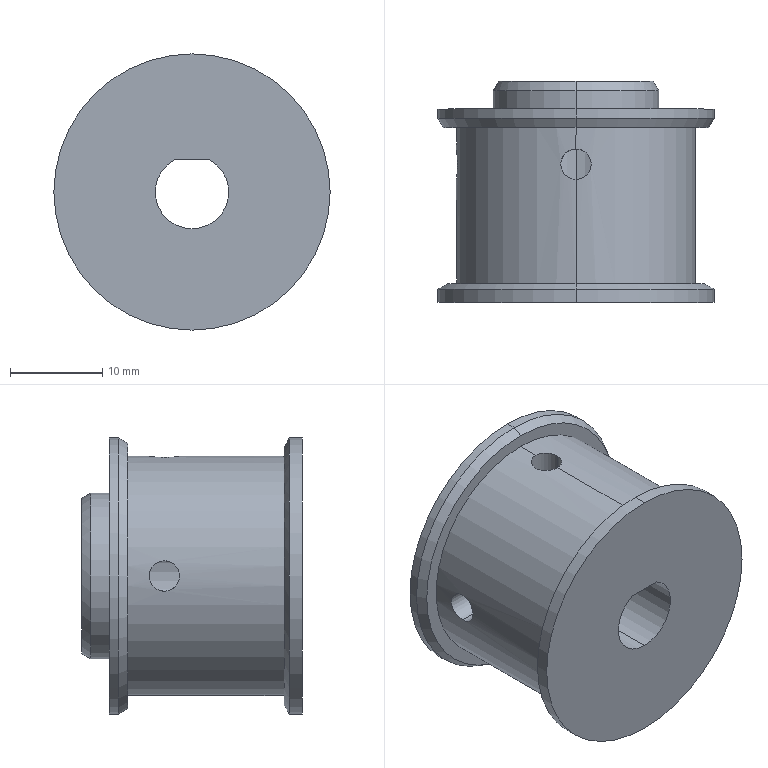Part | SolidWorks | features ICE 11, Chamfer 4, CirPattern 1, HoleWzd 1, Revolution 1 | 1 solid | 26 faces | box 30 x 24 x 30 mm | volume 11200 mm3 | cylinder 14 | cone 6 | plane 6 | commonest cylinder face diameters 3.3 x4 30 x4 8 x2 18 x2 25.98 x2
STEP:
#1=CARTESIAN_POINT('',(0.,24.,8.423));
#2=VERTEX_POINT('',#1);
#3=CARTESIAN_POINT('',(0.,24.,-8.423));
#4=VERTEX_POINT('',#3);
#5=CARTESIAN_POINT('',(0.,24.,0.));
#6=DIRECTION('',(0.,1.,0.));
#7=DIRECTION('',(0.,0.,1.));
#8=AXIS2_PLACEMENT_3D('',#5,#6,#7);
#9=CIRCLE('',#8,8.423);
#10=EDGE_CURVE('',#2,#4,#9,.T.);
#11=ORIENTED_EDGE('',*,*,#10,.F.);
#12=CARTESIAN_POINT('',(0.,23.,9.));
#13=VERTEX_POINT('',#12);
#14=CARTESIAN_POINT('',(0.,24.,8.423));
#15=DIRECTION('',(0.,-0.866,0.5));
#16=VECTOR('',#15,1000.);
#17=LINE('',#14,#16);
#18=EDGE_CURVE('',#2,#13,#17,.T.);
#19=ORIENTED_EDGE('',*,*,#18,.T.);
#20=CARTESIAN_POINT('',(0.,23.,-9.));
#21=VERTEX_POINT('',#20);
#22=CARTESIAN_POINT('',(0.,23.,0.));
#23=DIRECTION('',(0.,-1.,0.));
#24=DIRECTION('',(0.,0.,1.));
#25=AXIS2_PLACEMENT_3D('',#22,#23,#24);
#26=CIRCLE('',#25,9.);
#27=EDGE_CURVE('',#21,#13,#26,.T.);
#28=ORIENTED_EDGE('',*,*,#27,.F.);
#29=CARTESIAN_POINT('',(0.,24.,-8.423));
#30=DIRECTION('',(0.,-0.866,-0.5));
#31=VECTOR('',#30,1000.);
#32=LINE('',#29,#31);
#33=EDGE_CURVE('',#4,#21,#32,.T.);
#34=ORIENTED_EDGE('',*,*,#33,.F.);
#35=EDGE_LOOP('',(#11,#19,#28,#34));
#36=FACE_OUTER_BOUND('',#35,.T.);
#37=CARTESIAN_POINT('',(0.,24.,0.));
#38=DIRECTION('',(0.,-1.,0.));
#39=DIRECTION('',(0.,0.,-1.));
#40=AXIS2_PLACEMENT_3D('',#37,#38,#39);
#41=CONICAL_SURFACE('',#40,8.423,0.5236);
#42=ADVANCED_FACE('',(#36),#41,.T.);
#43=CARTESIAN_POINT('',(-12.885,15.,-1.65));
#44=VERTEX_POINT('',#43);
#45=CARTESIAN_POINT('',(-12.885,15.,1.65));
#46=VERTEX_POINT('',#45);
#47=CARTESIAN_POINT('',(-12.885,15.,-1.65));
#48=CARTESIAN_POINT('',(-12.885,14.891,-1.65));
#49=CARTESIAN_POINT('',(-12.886,14.784,-1.639));
#50=CARTESIAN_POINT('',(-12.891,14.573,-1.597));
#51=CARTESIAN_POINT('',(-12.895,14.468,-1.566));
#52=CARTESIAN_POINT('',(-12.905,14.268,-1.483));
#53=CARTESIAN_POINT('',(-12.911,14.173,-1.432));
#54=CARTESIAN_POINT('',(-12.924,13.994,-1.312));
#55=CARTESIAN_POINT('',(-12.931,13.909,-1.243));
#56=CARTESIAN_POINT('',(-12.951,13.681,-1.014));
#57=CARTESIAN_POINT('',(-12.965,13.558,-0.8305));
#58=CARTESIAN_POINT('',(-12.984,13.393,-0.4334));
#59=CARTESIAN_POINT('',(-12.99,13.35,-0.2161));
#60=CARTESIAN_POINT('',(-12.99,13.35,0.1071));
#61=CARTESIAN_POINT('',(-12.989,13.361,0.2166));
#62=CARTESIAN_POINT('',(-12.983,13.403,0.4283));
#63=CARTESIAN_POINT('',(-12.98,13.434,0.5312));
#64=CARTESIAN_POINT('',(-12.97,13.517,0.7311));
#65=CARTESIAN_POINT('',(-12.964,13.569,0.8276));
#66=CARTESIAN_POINT('',(-12.951,13.688,1.006));
#67=CARTESIAN_POINT('',(-12.944,13.756,1.09));
#68=CARTESIAN_POINT('',(-12.931,13.91,1.244));
#69=CARTESIAN_POINT('',(-12.924,13.993,1.312));
#70=CARTESIAN_POINT('',(-12.911,14.172,1.431));
#71=CARTESIAN_POINT('',(-12.905,14.269,1.483));
#72=CARTESIAN_POINT('',(-12.895,14.468,1.566));
#73=CARTESIAN_POINT('',(-12.891,14.571,1.597));
#74=CARTESIAN_POINT('',(-12.886,14.783,1.639));
#75=CARTESIAN_POINT('',(-12.885,14.892,1.65));
#76=CARTESIAN_POINT('',(-12.885,15.,1.65));
#77=B_SPLINE_CURVE_WITH_KNOTS('',3,(#47,#48,#49,#50,#51,#52,#53,#54,#55,#56,#57,#58,#59,#60,#61,#62,#63,#64,#65,#66,#67,#68,#69,#70,#71,#72,#73,#74,#75,#76),.UNSPECIFIED.,.F.,.F.,(4,2,2,2,2,2,2,2,2,2,2,2,2,2,4),(0.,0.0003227,0.0006455,0.0009682,0.001291,0.001936,0.002582,0.002905,0.003227,0.00355,0.003873,0.004196,0.004518,0.004841,0.005164),.UNSPECIFIED.);
#78=EDGE_CURVE('',#44,#46,#77,.T.);
#79=ORIENTED_EDGE('',*,*,#78,.T.);
#80=CARTESIAN_POINT('',(-3.644,15.,1.65));
#81=VERTEX_POINT('',#80);
#82=CARTESIAN_POINT('',(0.,15.,1.65));
#83=DIRECTION('',(1.,0.,0.));
#84=VECTOR('',#83,1000.);
#85=LINE('',#82,#84);
#86=EDGE_CURVE('',#46,#81,#85,.T.);
#87=ORIENTED_EDGE('',*,*,#86,.T.);
#88=CARTESIAN_POINT('',(-3.644,15.,-1.65));
#89=VERTEX_POINT('',#88);
#90=CARTESIAN_POINT('',(-3.644,15.,1.65));
#91=CARTESIAN_POINT('',(-3.644,14.891,1.65));
#92=CARTESIAN_POINT('',(-3.649,14.781,1.639));
#93=CARTESIAN_POINT('',(-3.668,14.568,1.596));
#94=CARTESIAN_POINT('',(-3.682,14.464,1.564));
#95=CARTESIAN_POINT('',(-3.733,14.165,1.439));
#96=CARTESIAN_POINT('',(-3.78,13.985,1.318));
#97=CARTESIAN_POINT('',(-3.849,13.757,1.091));
#98=CARTESIAN_POINT('',(-3.872,13.69,1.008));
#99=CARTESIAN_POINT('',(-3.914,13.571,0.8311));
#100=CARTESIAN_POINT('',(-3.933,13.519,0.7348));
#101=CARTESIAN_POINT('',(-3.965,13.436,0.5356));
#102=CARTESIAN_POINT('',(-3.978,13.404,0.4326));
#103=CARTESIAN_POINT('',(-3.995,13.361,0.2196));
#104=CARTESIAN_POINT('',(-4.,13.35,0.109));
#105=CARTESIAN_POINT('',(-4.,13.35,-0.2173));
#106=CARTESIAN_POINT('',(-3.981,13.394,-0.4365));
#107=CARTESIAN_POINT('',(-3.933,13.519,-0.7349));
#108=CARTESIAN_POINT('',(-3.914,13.571,-0.8311));
#109=CARTESIAN_POINT('',(-3.872,13.69,-1.009));
#110=CARTESIAN_POINT('',(-3.849,13.758,-1.091));
#111=CARTESIAN_POINT('',(-3.803,13.909,-1.243));
#112=CARTESIAN_POINT('',(-3.78,13.993,-1.311));
#113=CARTESIAN_POINT('',(-3.736,14.17,-1.43));
#114=CARTESIAN_POINT('',(-3.716,14.264,-1.481));
#115=CARTESIAN_POINT('',(-3.664,14.565,-1.607));
#116=CARTESIAN_POINT('',(-3.644,14.779,-1.65));
#117=CARTESIAN_POINT('',(-3.644,15.,-1.65));
#118=B_SPLINE_CURVE_WITH_KNOTS('',3,(#90,#91,#92,#93,#94,#95,#96,#97,#98,#99,#100,#101,#102,#103,#104,#105,#106,#107,#108,#109,#110,#111,#112,#113,#114,#115,#116,#117),.UNSPECIFIED.,.F.,.F.,(4,2,2,2,2,2,2,2,2,2,2,2,2,4),(0.005217,0.005543,0.005869,0.006521,0.006846,0.007172,0.007498,0.007824,0.008476,0.008801,0.009127,0.009453,0.009779,0.01043),.UNSPECIFIED.);
#119=EDGE_CURVE('',#81,#89,#118,.T.);
#120=ORIENTED_EDGE('',*,*,#119,.T.);
#121=CARTESIAN_POINT('',(0.,15.,-1.65));
#122=DIRECTION('',(1.,0.,0.));
#123=VECTOR('',#122,1000.);
#124=LINE('',#121,#123);
#125=EDGE_CURVE('',#44,#89,#124,.T.);
#126=ORIENTED_EDGE('',*,*,#125,.F.);
#127=EDGE_LOOP('',(#79,#87,#120,#126));
#128=FACE_OUTER_BOUND('',#127,.T.);
#129=CARTESIAN_POINT('',(0.,15.,0.));
#130=DIRECTION('',(1.,0.,0.));
#131=DIRECTION('',(0.,0.,-1.));
#132=AXIS2_PLACEMENT_3D('',#129,#130,#131);
#133=CYLINDRICAL_SURFACE('',#132,1.65);
#134=ADVANCED_FACE('',(#128),#133,.F.);
#135=CARTESIAN_POINT('',(0.,13.35,12.99));
#136=VERTEX_POINT('',#135);
#137=CARTESIAN_POINT('',(1.65,15.,12.885));
#138=VERTEX_POINT('',#137);
#139=CARTESIAN_POINT('',(0.,13.35,12.99));
#140=CARTESIAN_POINT('',(0.1077,13.35,12.99));
#141=CARTESIAN_POINT('',(0.2171,13.361,12.989));
#142=CARTESIAN_POINT('',(0.4288,13.403,12.983));
#143=CARTESIAN_POINT('',(0.5317,13.434,12.98));
#144=CARTESIAN_POINT('',(0.7315,13.517,12.97));
#145=CARTESIAN_POINT('',(0.8279,13.569,12.964));
#146=CARTESIAN_POINT('',(1.007,13.688,12.951));
#147=CARTESIAN_POINT('',(1.09,13.756,12.944));
#148=CARTESIAN_POINT('',(1.244,13.91,12.931));
#149=CARTESIAN_POINT('',(1.312,13.994,12.924));
#150=CARTESIAN_POINT('',(1.431,14.172,12.911));
#151=CARTESIAN_POINT('',(1.483,14.269,12.905));
#152=CARTESIAN_POINT('',(1.566,14.468,12.895));
#153=CARTESIAN_POINT('',(1.597,14.571,12.891));
#154=CARTESIAN_POINT('',(1.639,14.783,12.886));
#155=CARTESIAN_POINT('',(1.65,14.892,12.885));
#156=CARTESIAN_POINT('',(1.65,15.,12.885));
#157=B_SPLINE_CURVE_WITH_KNOTS('',3,(#139,#140,#141,#142,#143,#144,#145,#146,#147,#148,#149,#150,#151,#152,#153,#154,#155,#156),.UNSPECIFIED.,.F.,.F.,(4,2,2,2,2,2,2,2,4),(0.002583,0.002905,0.003228,0.003551,0.003873,0.004196,0.004519,0.004841,0.005164),.UNSPECIFIED.);
#158=EDGE_CURVE('',#136,#138,#157,.T.);
#159=ORIENTED_EDGE('',*,*,#158,.T.);
#160=CARTESIAN_POINT('',(1.65,15.,3.5));
#161=VERTEX_POINT('',#160);
#162=CARTESIAN_POINT('',(1.65,15.,0.));
#163=DIRECTION('',(0.,0.,-1.));
#164=VECTOR('',#163,1000.);
#165=LINE('',#162,#164);
#166=EDGE_CURVE('',#138,#161,#165,.T.);
#167=ORIENTED_EDGE('',*,*,#166,.T.);
#168=CARTESIAN_POINT('',(-1.65,15.,3.5));
#169=VERTEX_POINT('',#168);
#170=CARTESIAN_POINT('',(0.,15.,3.5));
#171=DIRECTION('',(0.,0.,-1.));
#172=DIRECTION('',(-1.,0.,0.));
#173=AXIS2_PLACEMENT_3D('',#170,#171,#172);
#174=CIRCLE('',#173,1.65);
#175=EDGE_CURVE('',#161,#169,#174,.T.);
#176=ORIENTED_EDGE('',*,*,#175,.T.);
#177=CARTESIAN_POINT('',(-1.65,15.,12.885));
#178=VERTEX_POINT('',#177);
#179=CARTESIAN_POINT('',(-1.65,15.,0.));
#180=DIRECTION('',(0.,0.,-1.));
#181=VECTOR('',#180,1000.);
#182=LINE('',#179,#181);
#183=EDGE_CURVE('',#178,#169,#182,.T.);
#184=ORIENTED_EDGE('',*,*,#183,.F.);
#185=CARTESIAN_POINT('',(-1.65,15.,12.885));
#186=CARTESIAN_POINT('',(-1.65,14.891,12.885));
#187=CARTESIAN_POINT('',(-1.639,14.784,12.886));
#188=CARTESIAN_POINT('',(-1.597,14.572,12.891));
#189=CARTESIAN_POINT('',(-1.565,14.468,12.895));
#190=CARTESIAN_POINT('',(-1.483,14.268,12.905));
#191=CARTESIAN_POINT('',(-1.432,14.173,12.911));
#192=CARTESIAN_POINT('',(-1.312,13.994,12.924));
#193=CARTESIAN_POINT('',(-1.242,13.909,12.931));
#194=CARTESIAN_POINT('',(-1.014,13.681,12.951));
#195=CARTESIAN_POINT('',(-0.8301,13.558,12.965));
#196=CARTESIAN_POINT('',(-0.4329,13.393,12.984));
#197=CARTESIAN_POINT('',(-0.2155,13.35,12.99));
#198=CARTESIAN_POINT('',(0.,13.35,12.99));
#199=B_SPLINE_CURVE_WITH_KNOTS('',3,(#185,#186,#187,#188,#189,#190,#191,#192,#193,#194,#195,#196,#197,#198),.UNSPECIFIED.,.F.,.F.,(4,2,2,2,2,2,4),(0.,0.0003228,0.0006456,0.0009685,0.001291,0.001937,0.002583),.UNSPECIFIED.);
#200=EDGE_CURVE('',#178,#136,#199,.T.);
#201=ORIENTED_EDGE('',*,*,#200,.T.);
#202=EDGE_LOOP('',(#159,#167,#176,#184,#201));
#203=FACE_OUTER_BOUND('',#202,.T.);
#204=CARTESIAN_POINT('',(0.,15.,0.));
#205=DIRECTION('',(0.,0.,-1.));
#206=DIRECTION('',(-1.,0.,0.));
#207=AXIS2_PLACEMENT_3D('',#204,#205,#206);
#208=CYLINDRICAL_SURFACE('',#207,1.65);
#209=ADVANCED_FACE('',(#203),#208,.F.);
#210=CARTESIAN_POINT('',(0.,2.,14.));
#211=VERTEX_POINT('',#210);
#212=CARTESIAN_POINT('',(0.,2.,-14.));
#213=VERTEX_POINT('',#212);
#214=CARTESIAN_POINT('',(0.,2.,0.));
#215=DIRECTION('',(0.,1.,0.));
#216=DIRECTION('',(0.,0.,1.));
#217=AXIS2_PLACEMENT_3D('',#214,#215,#216);
#218=CIRCLE('',#217,14.);
#219=EDGE_CURVE('',#211,#213,#218,.T.);
#220=ORIENTED_EDGE('',*,*,#219,.F.);
#221=CARTESIAN_POINT('',(0.,1.423,15.));
#222=VERTEX_POINT('',#221);
#223=CARTESIAN_POINT('',(0.,1.423,15.));
#224=DIRECTION('',(0.,-0.5,0.866));
#225=VECTOR('',#224,1000.);
#226=LINE('',#223,#225);
#227=EDGE_CURVE('',#211,#222,#226,.T.);
#228=ORIENTED_EDGE('',*,*,#227,.T.);
#229=CARTESIAN_POINT('',(0.,1.423,-15.));
#230=VERTEX_POINT('',#229);
#231=CARTESIAN_POINT('',(0.,1.423,0.));
#232=DIRECTION('',(0.,-1.,0.));
#233=DIRECTION('',(0.,0.,1.));
#234=AXIS2_PLACEMENT_3D('',#231,#232,#233);
#235=CIRCLE('',#234,15.);
#236=EDGE_CURVE('',#230,#222,#235,.T.);
#237=ORIENTED_EDGE('',*,*,#236,.F.);
#238=CARTESIAN_POINT('',(0.,1.423,-15.));
#239=DIRECTION('',(0.,-0.5,-0.866));
#240=VECTOR('',#239,1000.);
#241=LINE('',#238,#240);
#242=EDGE_CURVE('',#213,#230,#241,.T.);
#243=ORIENTED_EDGE('',*,*,#242,.F.);
#244=EDGE_LOOP('',(#220,#228,#237,#243));
#245=FACE_OUTER_BOUND('',#244,.T.);
#246=CARTESIAN_POINT('',(0.,1.423,0.));
#247=DIRECTION('',(0.,-1.,0.));
#248=DIRECTION('',(0.,0.,-1.));
#249=AXIS2_PLACEMENT_3D('',#246,#247,#248);
#250=CONICAL_SURFACE('',#249,15.,1.047);
#251=ADVANCED_FACE('',(#245),#250,.T.);
#252=CARTESIAN_POINT('',(0.,19.,-14.423));
#253=VERTEX_POINT('',#252);
#254=CARTESIAN_POINT('',(0.,19.,14.423));
#255=VERTEX_POINT('',#254);
#256=CARTESIAN_POINT('',(0.,19.,0.));
#257=DIRECTION('',(0.,-1.,0.));
#258=DIRECTION('',(0.,0.,-1.));
#259=AXIS2_PLACEMENT_3D('',#256,#257,#258);
#260=CIRCLE('',#259,14.423);
#261=EDGE_CURVE('',#253,#255,#260,.T.);
#262=ORIENTED_EDGE('',*,*,#261,.F.);
#263=CARTESIAN_POINT('',(0.,20.,-15.));
#264=VERTEX_POINT('',#263);
#265=CARTESIAN_POINT('',(0.,19.,-14.423));
#266=DIRECTION('',(0.,0.866,-0.5));
#267=VECTOR('',#266,1000.);
#268=LINE('',#265,#267);
#269=EDGE_CURVE('',#253,#264,#268,.T.);
#270=ORIENTED_EDGE('',*,*,#269,.T.);
#271=CARTESIAN_POINT('',(0.,20.,15.));
#272=VERTEX_POINT('',#271);
#273=CARTESIAN_POINT('',(0.,20.,0.));
#274=DIRECTION('',(0.,1.,0.));
#275=DIRECTION('',(0.,0.,-1.));
#276=AXIS2_PLACEMENT_3D('',#273,#274,#275);
#277=CIRCLE('',#276,15.);
#278=EDGE_CURVE('',#272,#264,#277,.T.);
#279=ORIENTED_EDGE('',*,*,#278,.F.);
#280=CARTESIAN_POINT('',(0.,19.,14.423));
#281=DIRECTION('',(0.,0.866,0.5));
#282=VECTOR('',#281,1000.);
#283=LINE('',#280,#282);
#284=EDGE_CURVE('',#255,#272,#283,.T.);
#285=ORIENTED_EDGE('',*,*,#284,.F.);
#286=EDGE_LOOP('',(#262,#270,#279,#285));
#287=FACE_OUTER_BOUND('',#286,.T.);
#288=CARTESIAN_POINT('',(0.,19.,0.));
#289=DIRECTION('',(0.,1.,0.));
#290=DIRECTION('',(0.,0.,1.));
#291=AXIS2_PLACEMENT_3D('',#288,#289,#290);
#292=CONICAL_SURFACE('',#291,14.423,0.5236);
#293=ADVANCED_FACE('',(#287),#292,.T.);
#294=CARTESIAN_POINT('',(0.,19.,-12.99));
#295=VERTEX_POINT('',#294);
#296=CARTESIAN_POINT('',(0.,19.,12.99));
#297=VERTEX_POINT('',#296);
#298=CARTESIAN_POINT('',(0.,19.,0.));
#299=DIRECTION('',(0.,-1.,0.));
#300=DIRECTION('',(0.,0.,-1.));
#301=AXIS2_PLACEMENT_3D('',#298,#299,#300);
#302=CIRCLE('',#301,12.99);
#303=EDGE_CURVE('',#295,#297,#302,.T.);
#304=ORIENTED_EDGE('',*,*,#303,.T.);
#305=CARTESIAN_POINT('',(0.,16.65,12.99));
#306=VERTEX_POINT('',#305);
#307=CARTESIAN_POINT('',(0.,0.,12.99));
#308=DIRECTION('',(0.,-1.,0.));
#309=VECTOR('',#308,1000.);
#310=LINE('',#307,#309);
#311=EDGE_CURVE('',#297,#306,#310,.T.);
#312=ORIENTED_EDGE('',*,*,#311,.T.);
#313=CARTESIAN_POINT('',(1.65,15.,12.885));
#314=CARTESIAN_POINT('',(1.65,15.216,12.885));
#315=CARTESIAN_POINT('',(1.607,15.433,12.891));
#316=CARTESIAN_POINT('',(1.442,15.83,12.91));
#317=CARTESIAN_POINT('',(1.319,16.014,12.924));
#318=CARTESIAN_POINT('',(1.091,16.242,12.944));
#319=CARTESIAN_POINT('',(1.006,16.312,12.951));
#320=CARTESIAN_POINT('',(0.827,16.432,12.964));
#321=CARTESIAN_POINT('',(0.7323,16.483,12.97));
#322=CARTESIAN_POINT('',(0.5324,16.565,12.979));
#323=CARTESIAN_POINT('',(0.4276,16.597,12.983));
#324=CARTESIAN_POINT('',(0.2165,16.639,12.989));
#325=CARTESIAN_POINT('',(0.1091,16.65,12.99));
#326=CARTESIAN_POINT('',(0.,16.65,12.99));
#327=B_SPLINE_CURVE_WITH_KNOTS('',3,(#313,#314,#315,#316,#317,#318,#319,#320,#321,#322,#323,#324,#325,#326),.UNSPECIFIED.,.F.,.F.,(4,2,2,2,2,2,4),(0.005164,0.005809,0.006455,0.006778,0.007101,0.007424,0.007746),.UNSPECIFIED.);
#328=EDGE_CURVE('',#138,#306,#327,.T.);
#329=ORIENTED_EDGE('',*,*,#328,.F.);
#330=ORIENTED_EDGE('',*,*,#158,.F.);
#331=CARTESIAN_POINT('',(0.,2.,12.99));
#332=VERTEX_POINT('',#331);
#333=CARTESIAN_POINT('',(0.,0.,12.99));
#334=DIRECTION('',(0.,-1.,0.));
#335=VECTOR('',#334,1000.);
#336=LINE('',#333,#335);
#337=EDGE_CURVE('',#136,#332,#336,.T.);
#338=ORIENTED_EDGE('',*,*,#337,.T.);
#339=CARTESIAN_POINT('',(0.,2.,-12.99));
#340=VERTEX_POINT('',#339);
#341=CARTESIAN_POINT('',(0.,2.,0.));
#342=DIRECTION('',(0.,-1.,0.));
#343=DIRECTION('',(0.,0.,-1.));
#344=AXIS2_PLACEMENT_3D('',#341,#342,#343);
#345=CIRCLE('',#344,12.99);
#346=EDGE_CURVE('',#340,#332,#345,.T.);
#347=ORIENTED_EDGE('',*,*,#346,.F.);
#348=CARTESIAN_POINT('',(0.,0.,-12.99));
#349=DIRECTION('',(0.,-1.,0.));
#350=VECTOR('',#349,1000.);
#351=LINE('',#348,#350);
#352=EDGE_CURVE('',#295,#340,#351,.T.);
#353=ORIENTED_EDGE('',*,*,#352,.F.);
#354=EDGE_LOOP('',(#304,#312,#329,#330,#338,#347,#353));
#355=FACE_OUTER_BOUND('',#354,.T.);
#356=CARTESIAN_POINT('',(0.,0.,0.));
#357=DIRECTION('',(0.,-1.,0.));
#358=DIRECTION('',(0.,0.,-1.));
#359=AXIS2_PLACEMENT_3D('',#356,#357,#358);
#360=CYLINDRICAL_SURFACE('',#359,12.99);
#361=ADVANCED_FACE('',(#355),#360,.T.);
#362=ORIENTED_EDGE('',*,*,#236,.T.);
#363=CARTESIAN_POINT('',(0.,0.,15.));
#364=VERTEX_POINT('',#363);
#365=CARTESIAN_POINT('',(0.,0.,15.));
#366=DIRECTION('',(0.,-1.,0.));
#367=VECTOR('',#366,1000.);
#368=LINE('',#365,#367);
#369=EDGE_CURVE('',#222,#364,#368,.T.);
#370=ORIENTED_EDGE('',*,*,#369,.T.);
#371=CARTESIAN_POINT('',(0.,0.,-15.));
#372=VERTEX_POINT('',#371);
#373=CARTESIAN_POINT('',(0.,0.,0.));
#374=DIRECTION('',(0.,-1.,0.));
#375=DIRECTION('',(0.,0.,-1.));
#376=AXIS2_PLACEMENT_3D('',#373,#374,#375);
#377=CIRCLE('',#376,15.);
#378=EDGE_CURVE('',#372,#364,#377,.T.);
#379=ORIENTED_EDGE('',*,*,#378,.F.);
#380=CARTESIAN_POINT('',(0.,0.,-15.));
#381=DIRECTION('',(0.,-1.,0.));
#382=VECTOR('',#381,1000.);
#383=LINE('',#380,#382);
#384=EDGE_CURVE('',#230,#372,#383,.T.);
#385=ORIENTED_EDGE('',*,*,#384,.F.);
#386=EDGE_LOOP('',(#362,#370,#379,#385));
#387=FACE_OUTER_BOUND('',#386,.T.);
#388=CARTESIAN_POINT('',(0.,0.,0.));
#389=DIRECTION('',(0.,-1.,0.));
#390=DIRECTION('',(0.,0.,-1.));
#391=AXIS2_PLACEMENT_3D('',#388,#389,#390);
#392=CYLINDRICAL_SURFACE('',#391,15.);
#393=ADVANCED_FACE('',(#387),#392,.T.);
#394=CARTESIAN_POINT('',(0.,21.,15.));
#395=VERTEX_POINT('',#394);
#396=CARTESIAN_POINT('',(0.,21.,-15.));
#397=VERTEX_POINT('',#396);
#398=CARTESIAN_POINT('',(0.,21.,0.));
#399=DIRECTION('',(0.,1.,0.));
#400=DIRECTION('',(0.,0.,1.));
#401=AXIS2_PLACEMENT_3D('',#398,#399,#400);
#402=CIRCLE('',#401,15.);
#403=EDGE_CURVE('',#395,#397,#402,.T.);
#404=ORIENTED_EDGE('',*,*,#403,.F.);
#405=CARTESIAN_POINT('',(0.,0.,15.));
#406=DIRECTION('',(0.,-1.,0.));
#407=VECTOR('',#406,1000.);
#408=LINE('',#405,#407);
#409=EDGE_CURVE('',#395,#272,#408,.T.);
#410=ORIENTED_EDGE('',*,*,#409,.T.);
#411=ORIENTED_EDGE('',*,*,#278,.T.);
#412=CARTESIAN_POINT('',(0.,0.,-15.));
#413=DIRECTION('',(0.,-1.,0.));
#414=VECTOR('',#413,1000.);
#415=LINE('',#412,#414);
#416=EDGE_CURVE('',#397,#264,#415,.T.);
#417=ORIENTED_EDGE('',*,*,#416,.F.);
#418=EDGE_LOOP('',(#404,#410,#411,#417));
#419=FACE_OUTER_BOUND('',#418,.T.);
#420=CARTESIAN_POINT('',(0.,0.,0.));
#421=DIRECTION('',(0.,-1.,0.));
#422=DIRECTION('',(0.,0.,-1.));
#423=AXIS2_PLACEMENT_3D('',#420,#421,#422);
#424=CYLINDRICAL_SURFACE('',#423,15.);
#425=ADVANCED_FACE('',(#419),#424,.T.);
#426=ORIENTED_EDGE('',*,*,#27,.T.);
#427=CARTESIAN_POINT('',(0.,21.,9.));
#428=VERTEX_POINT('',#427);
#429=CARTESIAN_POINT('',(0.,29.,9.));
#430=DIRECTION('',(0.,-1.,0.));
#431=VECTOR('',#430,1000.);
#432=LINE('',#429,#431);
#433=EDGE_CURVE('',#13,#428,#432,.T.);
#434=ORIENTED_EDGE('',*,*,#433,.T.);
#435=CARTESIAN_POINT('',(0.,21.,-9.));
#436=VERTEX_POINT('',#435);
#437=CARTESIAN_POINT('',(0.,21.,0.));
#438=DIRECTION('',(0.,1.,0.));
#439=DIRECTION('',(0.,0.,1.));
#440=AXIS2_PLACEMENT_3D('',#437,#438,#439);
#441=CIRCLE('',#440,9.);
#442=EDGE_CURVE('',#428,#436,#441,.T.);
#443=ORIENTED_EDGE('',*,*,#442,.T.);
#444=CARTESIAN_POINT('',(0.,29.,-9.));
#445=DIRECTION('',(0.,-1.,0.));
#446=VECTOR('',#445,1000.);
#447=LINE('',#444,#446);
#448=EDGE_CURVE('',#21,#436,#447,.T.);
#449=ORIENTED_EDGE('',*,*,#448,.F.);
#450=EDGE_LOOP('',(#426,#434,#443,#449));
#451=FACE_OUTER_BOUND('',#450,.T.);
#452=CARTESIAN_POINT('',(0.,29.,0.));
#453=DIRECTION('',(0.,-1.,0.));
#454=DIRECTION('',(0.,0.,-1.));
#455=AXIS2_PLACEMENT_3D('',#452,#453,#454);
#456=CYLINDRICAL_SURFACE('',#455,9.);
#457=ADVANCED_FACE('',(#451),#456,.T.);
#458=CARTESIAN_POINT('',(1.936,24.,3.5));
#459=VERTEX_POINT('',#458);
#460=CARTESIAN_POINT('',(0.,24.,-4.));
#461=VERTEX_POINT('',#460);
#462=CARTESIAN_POINT('',(0.,24.,0.));
#463=DIRECTION('',(0.,1.,0.));
#464=DIRECTION('',(0.,0.,1.));
#465=AXIS2_PLACEMENT_3D('',#462,#463,#464);
#466=CIRCLE('',#465,4.);
#467=EDGE_CURVE('',#459,#461,#466,.T.);
#468=ORIENTED_EDGE('',*,*,#467,.T.);
#469=CARTESIAN_POINT('',(0.,0.,-4.));
#470=VERTEX_POINT('',#469);
#471=CARTESIAN_POINT('',(0.,0.,-4.));
#472=DIRECTION('',(0.,-1.,0.));
#473=VECTOR('',#472,1000.);
#474=LINE('',#471,#473);
#475=EDGE_CURVE('',#461,#470,#474,.T.);
#476=ORIENTED_EDGE('',*,*,#475,.T.);
#477=CARTESIAN_POINT('',(1.936,0.,3.5));
#478=VERTEX_POINT('',#477);
#479=CARTESIAN_POINT('',(0.,0.,0.));
#480=DIRECTION('',(0.,-1.,0.));
#481=DIRECTION('',(0.,0.,-1.));
#482=AXIS2_PLACEMENT_3D('',#479,#480,#481);
#483=CIRCLE('',#482,4.);
#484=EDGE_CURVE('',#470,#478,#483,.T.);
#485=ORIENTED_EDGE('',*,*,#484,.T.);
#486=CARTESIAN_POINT('',(1.936,0.,3.5));
#487=DIRECTION('',(0.,1.,0.));
#488=VECTOR('',#487,1000.);
#489=LINE('',#486,#488);
#490=EDGE_CURVE('',#478,#459,#489,.T.);
#491=ORIENTED_EDGE('',*,*,#490,.T.);
#492=EDGE_LOOP('',(#468,#476,#485,#491));
#493=FACE_OUTER_BOUND('',#492,.T.);
#494=CARTESIAN_POINT('',(0.,0.,0.));
#495=DIRECTION('',(0.,-1.,0.));
#496=DIRECTION('',(0.,0.,-1.));
#497=AXIS2_PLACEMENT_3D('',#494,#495,#496);
#498=CYLINDRICAL_SURFACE('',#497,4.);
#499=ADVANCED_FACE('',(#493),#498,.F.);
#500=ORIENTED_EDGE('',*,*,#475,.F.);
#501=CARTESIAN_POINT('',(-1.936,24.,3.5));
#502=VERTEX_POINT('',#501);
#503=CARTESIAN_POINT('',(0.,24.,0.));
#504=DIRECTION('',(0.,1.,0.));
#505=DIRECTION('',(0.,0.,1.));
#506=AXIS2_PLACEMENT_3D('',#503,#504,#505);
#507=CIRCLE('',#506,4.);
#508=EDGE_CURVE('',#461,#502,#507,.T.);
#509=ORIENTED_EDGE('',*,*,#508,.T.);
#510=CARTESIAN_POINT('',(-1.936,0.,3.5));
#511=VERTEX_POINT('',#510);
#512=CARTESIAN_POINT('',(-1.936,0.,3.5));
#513=DIRECTION('',(0.,1.,0.));
#514=VECTOR('',#513,1000.);
#515=LINE('',#512,#514);
#516=EDGE_CURVE('',#511,#502,#515,.T.);
#517=ORIENTED_EDGE('',*,*,#516,.F.);
#518=CARTESIAN_POINT('',(0.,0.,0.));
#519=DIRECTION('',(0.,-1.,0.));
#520=DIRECTION('',(0.,0.,-1.));
#521=AXIS2_PLACEMENT_3D('',#518,#519,#520);
#522=CIRCLE('',#521,4.);
#523=EDGE_CURVE('',#511,#470,#522,.T.);
#524=ORIENTED_EDGE('',*,*,#523,.T.);
#525=EDGE_LOOP('',(#500,#509,#517,#524));
#526=FACE_OUTER_BOUND('',#525,.T.);
#527=CARTESIAN_POINT('',(-3.644,15.,-1.65));
#528=CARTESIAN_POINT('',(-3.644,15.11,-1.65));
#529=CARTESIAN_POINT('',(-3.649,15.219,-1.639));
#530=CARTESIAN_POINT('',(-3.668,15.431,-1.596));
#531=CARTESIAN_POINT('',(-3.682,15.536,-1.564));
#532=CARTESIAN_POINT('',(-3.733,15.835,-1.439));
#533=CARTESIAN_POINT('',(-3.78,16.016,-1.317));
#534=CARTESIAN_POINT('',(-3.872,16.317,-1.016));
#535=CARTESIAN_POINT('',(-3.917,16.44,-0.8343));
#536=CARTESIAN_POINT('',(-3.965,16.564,-0.5369));
#537=CARTESIAN_POINT('',(-3.978,16.596,-0.4316));
#538=CARTESIAN_POINT('',(-3.995,16.639,-0.2179));
#539=CARTESIAN_POINT('',(-4.,16.65,-0.11));
#540=CARTESIAN_POINT('',(-4.,16.65,0.1082));
#541=CARTESIAN_POINT('',(-3.995,16.639,0.2188));
#542=CARTESIAN_POINT('',(-3.978,16.596,0.4317));
#543=CARTESIAN_POINT('',(-3.965,16.564,0.5355));
#544=CARTESIAN_POINT('',(-3.933,16.48,0.7367));
#545=CARTESIAN_POINT('',(-3.914,16.429,0.8311));
#546=CARTESIAN_POINT('',(-3.872,16.31,1.009));
#547=CARTESIAN_POINT('',(-3.849,16.241,1.093));
#548=CARTESIAN_POINT('',(-3.803,16.09,1.243));
#549=CARTESIAN_POINT('',(-3.78,16.008,1.311));
#550=CARTESIAN_POINT('',(-3.736,15.83,1.43));
#551=CARTESIAN_POINT('',(-3.716,15.734,1.482));
#552=CARTESIAN_POINT('',(-3.665,15.437,1.606));
#553=CARTESIAN_POINT('',(-3.644,15.217,1.65));
#554=CARTESIAN_POINT('',(-3.644,15.,1.65));
#555=B_SPLINE_CURVE_WITH_KNOTS('',3,(#527,#528,#529,#530,#531,#532,#533,#534,#535,#536,#537,#538,#539,#540,#541,#542,#543,#544,#545,#546,#547,#548,#549,#550,#551,#552,#553,#554),.UNSPECIFIED.,.F.,.F.,(4,2,2,2,2,2,2,2,2,2,2,2,2,4),(0.,0.0003261,0.0006522,0.001304,0.001956,0.002283,0.002609,0.002935,0.003261,0.003587,0.003913,0.004239,0.004565,0.005217),.UNSPECIFIED.);
#556=EDGE_CURVE('',#89,#81,#555,.T.);
#557=ORIENTED_EDGE('',*,*,#556,.F.);
#558=ORIENTED_EDGE('',*,*,#119,.F.);
#559=EDGE_LOOP('',(#557,#558));
#560=FACE_BOUND('',#559,.T.);
#561=CARTESIAN_POINT('',(0.,0.,0.));
#562=DIRECTION('',(0.,-1.,0.));
#563=DIRECTION('',(0.,0.,-1.));
#564=AXIS2_PLACEMENT_3D('',#561,#562,#563);
#565=CYLINDRICAL_SURFACE('',#564,4.);
#566=ADVANCED_FACE('',(#526,#560),#565,.F.);
#567=ORIENTED_EDGE('',*,*,#433,.F.);
#568=CARTESIAN_POINT('',(0.,23.,0.));
#569=DIRECTION('',(0.,-1.,0.));
#570=DIRECTION('',(0.,0.,1.));
#571=AXIS2_PLACEMENT_3D('',#568,#569,#570);
#572=CIRCLE('',#571,9.);
#573=EDGE_CURVE('',#13,#21,#572,.T.);
#574=ORIENTED_EDGE('',*,*,#573,.T.);
#575=ORIENTED_EDGE('',*,*,#448,.T.);
#576=CARTESIAN_POINT('',(0.,21.,0.));
#577=DIRECTION('',(0.,1.,0.));
#578=DIRECTION('',(0.,0.,1.));
#579=AXIS2_PLACEMENT_3D('',#576,#577,#578);
#580=CIRCLE('',#579,9.);
#581=EDGE_CURVE('',#436,#428,#580,.T.);
#582=ORIENTED_EDGE('',*,*,#581,.T.);
#583=EDGE_LOOP('',(#567,#574,#575,#582));
#584=FACE_OUTER_BOUND('',#583,.T.);
#585=CARTESIAN_POINT('',(0.,29.,0.));
#586=DIRECTION('',(0.,-1.,0.));
#587=DIRECTION('',(0.,0.,-1.));
#588=AXIS2_PLACEMENT_3D('',#585,#586,#587);
#589=CYLINDRICAL_SURFACE('',#588,9.);
#590=ADVANCED_FACE('',(#584),#589,.T.);
#591=CARTESIAN_POINT('',(0.,15.,3.5));
#592=DIRECTION('',(0.,0.,-1.));
#593=DIRECTION('',(-1.,0.,0.));
#594=AXIS2_PLACEMENT_3D('',#591,#592,#593);
#595=CIRCLE('',#594,1.65);
#596=EDGE_CURVE('',#169,#161,#595,.T.);
#597=ORIENTED_EDGE('',*,*,#596,.F.);
#598=ORIENTED_EDGE('',*,*,#175,.F.);
#599=EDGE_LOOP('',(#597,#598));
#600=FACE_BOUND('',#599,.T.);
#601=ORIENTED_EDGE('',*,*,#516,.T.);
#602=CARTESIAN_POINT('',(-1.936,24.,3.5));
#603=DIRECTION('',(1.,0.,0.));
#604=VECTOR('',#603,1000.);
#605=LINE('',#602,#604);
#606=EDGE_CURVE('',#502,#459,#605,.T.);
#607=ORIENTED_EDGE('',*,*,#606,.T.);
#608=ORIENTED_EDGE('',*,*,#490,.F.);
#609=CARTESIAN_POINT('',(-1.936,0.,3.5));
#610=DIRECTION('',(-1.,0.,0.));
#611=VECTOR('',#610,1000.);
#612=LINE('',#609,#611);
#613=EDGE_CURVE('',#478,#511,#612,.T.);
#614=ORIENTED_EDGE('',*,*,#613,.T.);
#615=EDGE_LOOP('',(#601,#607,#608,#614));
#616=FACE_OUTER_BOUND('',#615,.T.);
#617=CARTESIAN_POINT('',(-1.936,0.,3.5));
#618=DIRECTION('',(0.,0.,-1.));
#619=DIRECTION('',(-1.,0.,0.));
#620=AXIS2_PLACEMENT_3D('',#617,#618,#619);
#621=PLANE('',#620);
#622=ADVANCED_FACE('',(#600,#616),#621,.T.);
#623=CARTESIAN_POINT('',(0.,21.,0.));
#624=DIRECTION('',(0.,1.,0.));
#625=DIRECTION('',(0.,0.,1.));
#626=AXIS2_PLACEMENT_3D('',#623,#624,#625);
#627=CIRCLE('',#626,15.);
#628=EDGE_CURVE('',#397,#395,#627,.T.);
#629=ORIENTED_EDGE('',*,*,#628,.T.);
#630=ORIENTED_EDGE('',*,*,#403,.T.);
#631=EDGE_LOOP('',(#629,#630));
#632=FACE_OUTER_BOUND('',#631,.T.);
#633=ORIENTED_EDGE('',*,*,#581,.F.);
#634=ORIENTED_EDGE('',*,*,#442,.F.);
#635=EDGE_LOOP('',(#633,#634));
#636=FACE_BOUND('',#635,.T.);
#637=CARTESIAN_POINT('',(0.,21.,0.));
#638=DIRECTION('',(0.,1.,0.));
#639=DIRECTION('',(0.,0.,1.));
#640=AXIS2_PLACEMENT_3D('',#637,#638,#639);
#641=PLANE('',#640);
#642=ADVANCED_FACE('',(#632,#636),#641,.T.);
#643=ORIENTED_EDGE('',*,*,#409,.F.);
#644=ORIENTED_EDGE('',*,*,#628,.F.);
#645=ORIENTED_EDGE('',*,*,#416,.T.);
#646=CARTESIAN_POINT('',(0.,20.,0.));
#647=DIRECTION('',(0.,1.,0.));
#648=DIRECTION('',(0.,0.,-1.));
#649=AXIS2_PLACEMENT_3D('',#646,#647,#648);
#650=CIRCLE('',#649,15.);
#651=EDGE_CURVE('',#264,#272,#650,.T.);
#652=ORIENTED_EDGE('',*,*,#651,.T.);
#653=EDGE_LOOP('',(#643,#644,#645,#652));
#654=FACE_OUTER_BOUND('',#653,.T.);
#655=CARTESIAN_POINT('',(0.,0.,0.));
#656=DIRECTION('',(0.,-1.,0.));
#657=DIRECTION('',(0.,0.,-1.));
#658=AXIS2_PLACEMENT_3D('',#655,#656,#657);
#659=CYLINDRICAL_SURFACE('',#658,15.);
#660=ADVANCED_FACE('',(#654),#659,.T.);
#661=ORIENTED_EDGE('',*,*,#369,.F.);
#662=CARTESIAN_POINT('',(0.,1.423,0.));
#663=DIRECTION('',(0.,-1.,0.));
#664=DIRECTION('',(0.,0.,1.));
#665=AXIS2_PLACEMENT_3D('',#662,#663,#664);
#666=CIRCLE('',#665,15.);
#667=EDGE_CURVE('',#222,#230,#666,.T.);
#668=ORIENTED_EDGE('',*,*,#667,.T.);
#669=ORIENTED_EDGE('',*,*,#384,.T.);
#670=CARTESIAN_POINT('',(0.,0.,0.));
#671=DIRECTION('',(0.,-1.,0.));
#672=DIRECTION('',(0.,0.,-1.));
#673=AXIS2_PLACEMENT_3D('',#670,#671,#672);
#674=CIRCLE('',#673,15.);
#675=EDGE_CURVE('',#364,#372,#674,.T.);
#676=ORIENTED_EDGE('',*,*,#675,.F.);
#677=EDGE_LOOP('',(#661,#668,#669,#676));
#678=FACE_OUTER_BOUND('',#677,.T.);
#679=CARTESIAN_POINT('',(0.,0.,0.));
#680=DIRECTION('',(0.,-1.,0.));
#681=DIRECTION('',(0.,0.,-1.));
#682=AXIS2_PLACEMENT_3D('',#679,#680,#681);
#683=CYLINDRICAL_SURFACE('',#682,15.);
#684=ADVANCED_FACE('',(#678),#683,.T.);
#685=CARTESIAN_POINT('',(0.,19.,0.));
#686=DIRECTION('',(0.,-1.,0.));
#687=DIRECTION('',(0.,0.,-1.));
#688=AXIS2_PLACEMENT_3D('',#685,#686,#687);
#689=CIRCLE('',#688,14.423);
#690=EDGE_CURVE('',#255,#253,#689,.T.);
#691=ORIENTED_EDGE('',*,*,#690,.T.);
#692=ORIENTED_EDGE('',*,*,#261,.T.);
#693=EDGE_LOOP('',(#691,#692));
#694=FACE_OUTER_BOUND('',#693,.T.);
#695=ORIENTED_EDGE('',*,*,#303,.F.);
#696=CARTESIAN_POINT('',(0.,19.,0.));
#697=DIRECTION('',(0.,-1.,0.));
#698=DIRECTION('',(0.,0.,-1.));
#699=AXIS2_PLACEMENT_3D('',#696,#697,#698);
#700=CIRCLE('',#699,12.99);
#701=EDGE_CURVE('',#297,#295,#700,.T.);
#702=ORIENTED_EDGE('',*,*,#701,.F.);
#703=EDGE_LOOP('',(#695,#702));
#704=FACE_BOUND('',#703,.T.);
#705=CARTESIAN_POINT('',(15.,19.,0.));
#706=DIRECTION('',(0.,-1.,0.));
#707=DIRECTION('',(0.,0.,-1.));
#708=AXIS2_PLACEMENT_3D('',#705,#706,#707);
#709=PLANE('',#708);
#710=ADVANCED_FACE('',(#694,#704),#709,.T.);
#711=ORIENTED_EDGE('',*,*,#311,.F.);
#712=ORIENTED_EDGE('',*,*,#701,.T.);
#713=ORIENTED_EDGE('',*,*,#352,.T.);
#714=CARTESIAN_POINT('',(0.,2.,0.));
#715=DIRECTION('',(0.,-1.,0.));
#716=DIRECTION('',(0.,0.,-1.));
#717=AXIS2_PLACEMENT_3D('',#714,#715,#716);
#718=CIRCLE('',#717,12.99);
#719=EDGE_CURVE('',#332,#340,#718,.T.);
#720=ORIENTED_EDGE('',*,*,#719,.F.);
#721=ORIENTED_EDGE('',*,*,#337,.F.);
#722=ORIENTED_EDGE('',*,*,#200,.F.);
#723=CARTESIAN_POINT('',(0.,16.65,12.99));
#724=CARTESIAN_POINT('',(-0.109,16.65,12.99));
#725=CARTESIAN_POINT('',(-0.2162,16.639,12.989));
#726=CARTESIAN_POINT('',(-0.4272,16.597,12.983));
#727=CARTESIAN_POINT('',(-0.532,16.566,12.979));
#728=CARTESIAN_POINT('',(-0.7316,16.483,12.97));
#729=CARTESIAN_POINT('',(-0.8263,16.432,12.964));
#730=CARTESIAN_POINT('',(-1.006,16.313,12.951));
#731=CARTESIAN_POINT('',(-1.09,16.243,12.944));
#732=CARTESIAN_POINT('',(-1.318,16.015,12.924));
#733=CARTESIAN_POINT('',(-1.441,15.831,12.91));
#734=CARTESIAN_POINT('',(-1.606,15.435,12.891));
#735=CARTESIAN_POINT('',(-1.65,15.218,12.885));
#736=CARTESIAN_POINT('',(-1.65,15.,12.885));
#737=B_SPLINE_CURVE_WITH_KNOTS('',3,(#723,#724,#725,#726,#727,#728,#729,#730,#731,#732,#733,#734,#735,#736),.UNSPECIFIED.,.F.,.F.,(4,2,2,2,2,2,4),(0.007746,0.008069,0.008391,0.008714,0.009036,0.009681,0.01033),.UNSPECIFIED.);
#738=EDGE_CURVE('',#306,#178,#737,.T.);
#739=ORIENTED_EDGE('',*,*,#738,.F.);
#740=EDGE_LOOP('',(#711,#712,#713,#720,#721,#722,#739));
#741=FACE_OUTER_BOUND('',#740,.T.);
#742=ORIENTED_EDGE('',*,*,#78,.F.);
#743=CARTESIAN_POINT('',(-12.885,15.,1.65));
#744=CARTESIAN_POINT('',(-12.885,15.215,1.65));
#745=CARTESIAN_POINT('',(-12.891,15.433,1.607));
#746=CARTESIAN_POINT('',(-12.91,15.83,1.442));
#747=CARTESIAN_POINT('',(-12.924,16.014,1.319));
#748=CARTESIAN_POINT('',(-12.944,16.242,1.092));
#749=CARTESIAN_POINT('',(-12.951,16.312,1.007));
#750=CARTESIAN_POINT('',(-12.964,16.431,0.8277));
#751=CARTESIAN_POINT('',(-12.97,16.482,0.733));
#752=CARTESIAN_POINT('',(-12.979,16.565,0.5333));
#753=CARTESIAN_POINT('',(-12.983,16.597,0.4285));
#754=CARTESIAN_POINT('',(-12.989,16.639,0.2176));
#755=CARTESIAN_POINT('',(-12.99,16.65,0.1103));
#756=CARTESIAN_POINT('',(-12.99,16.65,-0.1079));
#757=CARTESIAN_POINT('',(-12.989,16.639,-0.2152));
#758=CARTESIAN_POINT('',(-12.983,16.598,-0.4262));
#759=CARTESIAN_POINT('',(-12.98,16.566,-0.5311));
#760=CARTESIAN_POINT('',(-12.97,16.483,-0.7309));
#761=CARTESIAN_POINT('',(-12.964,16.433,-0.8257));
#762=CARTESIAN_POINT('',(-12.951,16.313,-1.005));
#763=CARTESIAN_POINT('',(-12.944,16.243,-1.09));
#764=CARTESIAN_POINT('',(-12.924,16.016,-1.318));
#765=CARTESIAN_POINT('',(-12.91,15.832,-1.441));
#766=CARTESIAN_POINT('',(-12.891,15.435,-1.606));
#767=CARTESIAN_POINT('',(-12.885,15.218,-1.65));
#768=CARTESIAN_POINT('',(-12.885,15.,-1.65));
#769=B_SPLINE_CURVE_WITH_KNOTS('',3,(#743,#744,#745,#746,#747,#748,#749,#750,#751,#752,#753,#754,#755,#756,#757,#758,#759,#760,#761,#762,#763,#764,#765,#766,#767,#768),.UNSPECIFIED.,.F.,.F.,(4,2,2,2,2,2,2,2,2,2,2,2,4),(0.005164,0.005809,0.006455,0.006777,0.0071,0.007423,0.007745,0.008068,0.008391,0.008713,0.009036,0.009681,0.01033),.UNSPECIFIED.);
#770=EDGE_CURVE('',#46,#44,#769,.T.);
#771=ORIENTED_EDGE('',*,*,#770,.F.);
#772=EDGE_LOOP('',(#742,#771));
#773=FACE_BOUND('',#772,.T.);
#774=CARTESIAN_POINT('',(0.,0.,0.));
#775=DIRECTION('',(0.,-1.,0.));
#776=DIRECTION('',(0.,0.,-1.));
#777=AXIS2_PLACEMENT_3D('',#774,#775,#776);
#778=CYLINDRICAL_SURFACE('',#777,12.99);
#779=ADVANCED_FACE('',(#741,#773),#778,.T.);
#780=CARTESIAN_POINT('',(0.,2.,0.));
#781=DIRECTION('',(0.,1.,0.));
#782=DIRECTION('',(0.,0.,1.));
#783=AXIS2_PLACEMENT_3D('',#780,#781,#782);
#784=CIRCLE('',#783,14.);
#785=EDGE_CURVE('',#213,#211,#784,.T.);
#786=ORIENTED_EDGE('',*,*,#785,.T.);
#787=ORIENTED_EDGE('',*,*,#219,.T.);
#788=EDGE_LOOP('',(#786,#787));
#789=FACE_OUTER_BOUND('',#788,.T.);
#790=ORIENTED_EDGE('',*,*,#346,.T.);
#791=ORIENTED_EDGE('',*,*,#719,.T.);
#792=EDGE_LOOP('',(#790,#791));
#793=FACE_BOUND('',#792,.T.);
#794=CARTESIAN_POINT('',(12.99,2.,0.));
#795=DIRECTION('',(0.,1.,0.));
#796=DIRECTION('',(0.,0.,1.));
#797=AXIS2_PLACEMENT_3D('',#794,#795,#796);
#798=PLANE('',#797);
#799=ADVANCED_FACE('',(#789,#793),#798,.T.);
#800=ORIENTED_EDGE('',*,*,#378,.T.);
#801=ORIENTED_EDGE('',*,*,#675,.T.);
#802=EDGE_LOOP('',(#800,#801));
#803=FACE_OUTER_BOUND('',#802,.T.);
#804=ORIENTED_EDGE('',*,*,#523,.F.);
#805=ORIENTED_EDGE('',*,*,#613,.F.);
#806=ORIENTED_EDGE('',*,*,#484,.F.);
#807=EDGE_LOOP('',(#804,#805,#806));
#808=FACE_BOUND('',#807,.T.);
#809=CARTESIAN_POINT('',(0.,0.,0.));
#810=DIRECTION('',(0.,-1.,0.));
#811=DIRECTION('',(0.,0.,-1.));
#812=AXIS2_PLACEMENT_3D('',#809,#810,#811);
#813=PLANE('',#812);
#814=ADVANCED_FACE('',(#803,#808),#813,.T.);
#815=ORIENTED_EDGE('',*,*,#269,.F.);
#816=ORIENTED_EDGE('',*,*,#690,.F.);
#817=ORIENTED_EDGE('',*,*,#284,.T.);
#818=ORIENTED_EDGE('',*,*,#651,.F.);
#819=EDGE_LOOP('',(#815,#816,#817,#818));
#820=FACE_OUTER_BOUND('',#819,.T.);
#821=CARTESIAN_POINT('',(0.,19.,0.));
#822=DIRECTION('',(0.,1.,0.));
#823=DIRECTION('',(0.,0.,1.));
#824=AXIS2_PLACEMENT_3D('',#821,#822,#823);
#825=CONICAL_SURFACE('',#824,14.423,0.5236);
#826=ADVANCED_FACE('',(#820),#825,.T.);
#827=ORIENTED_EDGE('',*,*,#227,.F.);
#828=ORIENTED_EDGE('',*,*,#785,.F.);
#829=ORIENTED_EDGE('',*,*,#242,.T.);
#830=ORIENTED_EDGE('',*,*,#667,.F.);
#831=EDGE_LOOP('',(#827,#828,#829,#830));
#832=FACE_OUTER_BOUND('',#831,.T.);
#833=CARTESIAN_POINT('',(0.,1.423,0.));
#834=DIRECTION('',(0.,-1.,0.));
#835=DIRECTION('',(0.,0.,-1.));
#836=AXIS2_PLACEMENT_3D('',#833,#834,#835);
#837=CONICAL_SURFACE('',#836,15.,1.047);
#838=ADVANCED_FACE('',(#832),#837,.T.);
#839=ORIENTED_EDGE('',*,*,#166,.F.);
#840=ORIENTED_EDGE('',*,*,#328,.T.);
#841=ORIENTED_EDGE('',*,*,#738,.T.);
#842=ORIENTED_EDGE('',*,*,#183,.T.);
#843=ORIENTED_EDGE('',*,*,#596,.T.);
#844=EDGE_LOOP('',(#839,#840,#841,#842,#843));
#845=FACE_OUTER_BOUND('',#844,.T.);
#846=CARTESIAN_POINT('',(0.,15.,0.));
#847=DIRECTION('',(0.,0.,-1.));
#848=DIRECTION('',(-1.,0.,0.));
#849=AXIS2_PLACEMENT_3D('',#846,#847,#848);
#850=CYLINDRICAL_SURFACE('',#849,1.65);
#851=ADVANCED_FACE('',(#845),#850,.F.);
#852=ORIENTED_EDGE('',*,*,#86,.F.);
#853=ORIENTED_EDGE('',*,*,#770,.T.);
#854=ORIENTED_EDGE('',*,*,#125,.T.);
#855=ORIENTED_EDGE('',*,*,#556,.T.);
#856=EDGE_LOOP('',(#852,#853,#854,#855));
#857=FACE_OUTER_BOUND('',#856,.T.);
#858=CARTESIAN_POINT('',(0.,15.,0.));
#859=DIRECTION('',(1.,0.,0.));
#860=DIRECTION('',(0.,0.,-1.));
#861=AXIS2_PLACEMENT_3D('',#858,#859,#860);
#862=CYLINDRICAL_SURFACE('',#861,1.65);
#863=ADVANCED_FACE('',(#857),#862,.F.);
#864=CARTESIAN_POINT('',(0.,24.,0.));
#865=DIRECTION('',(0.,1.,0.));
#866=DIRECTION('',(0.,0.,1.));
#867=AXIS2_PLACEMENT_3D('',#864,#865,#866);
#868=CIRCLE('',#867,8.423);
#869=EDGE_CURVE('',#4,#2,#868,.T.);
#870=ORIENTED_EDGE('',*,*,#869,.T.);
#871=ORIENTED_EDGE('',*,*,#10,.T.);
#872=EDGE_LOOP('',(#870,#871));
#873=FACE_OUTER_BOUND('',#872,.T.);
#874=ORIENTED_EDGE('',*,*,#606,.F.);
#875=ORIENTED_EDGE('',*,*,#508,.F.);
#876=ORIENTED_EDGE('',*,*,#467,.F.);
#877=EDGE_LOOP('',(#874,#875,#876));
#878=FACE_BOUND('',#877,.T.);
#879=CARTESIAN_POINT('',(0.,24.,0.));
#880=DIRECTION('',(0.,1.,0.));
#881=DIRECTION('',(0.,0.,1.));
#882=AXIS2_PLACEMENT_3D('',#879,#880,#881);
#883=PLANE('',#882);
#884=ADVANCED_FACE('',(#873,#878),#883,.T.);
#885=ORIENTED_EDGE('',*,*,#18,.F.);
#886=ORIENTED_EDGE('',*,*,#869,.F.);
#887=ORIENTED_EDGE('',*,*,#33,.T.);
#888=ORIENTED_EDGE('',*,*,#573,.F.);
#889=EDGE_LOOP('',(#885,#886,#887,#888));
#890=FACE_OUTER_BOUND('',#889,.T.);
#891=CARTESIAN_POINT('',(0.,24.,0.));
#892=DIRECTION('',(0.,-1.,0.));
#893=DIRECTION('',(0.,0.,-1.));
#894=AXIS2_PLACEMENT_3D('',#891,#892,#893);
#895=CONICAL_SURFACE('',#894,8.423,0.5236);
#896=ADVANCED_FACE('',(#890),#895,.T.);
#897=CLOSED_SHELL('',(#42,#134,#209,#251,#293,#361,#393,#425,#457,#499,#566,#590,#622,#642,#660,#684,#710,#779,#799,#814,#826,#838,#851,#863,#884,#896));
#898=MANIFOLD_SOLID_BREP('',#897);
#899=CARTESIAN_POINT('',(0.,0.,0.));
#900=DIRECTION('',(0.,0.,1.));
#901=DIRECTION('',(1.,0.,0.));
#902=AXIS2_PLACEMENT_3D('',#899,#900,#901);
#903=(LENGTH_UNIT()NAMED_UNIT(*)SI_UNIT(.MILLI.,.METRE.));
#904=UNCERTAINTY_MEASURE_WITH_UNIT(LENGTH_MEASURE(0.00001),#903,'','');
#905=(NAMED_UNIT(*)PLANE_ANGLE_UNIT()SI_UNIT($,.RADIAN.));
#906=(NAMED_UNIT(*)SI_UNIT($,.STERADIAN.)SOLID_ANGLE_UNIT());
#907=(GEOMETRIC_REPRESENTATION_CONTEXT(3)GLOBAL_UNCERTAINTY_ASSIGNED_CONTEXT((#904))GLOBAL_UNIT_ASSIGNED_CONTEXT((#903,#905,#906))REPRESENTATION_CONTEXT('',''));
#908=ADVANCED_BREP_SHAPE_REPRESENTATION('',(#898,#902),#907);